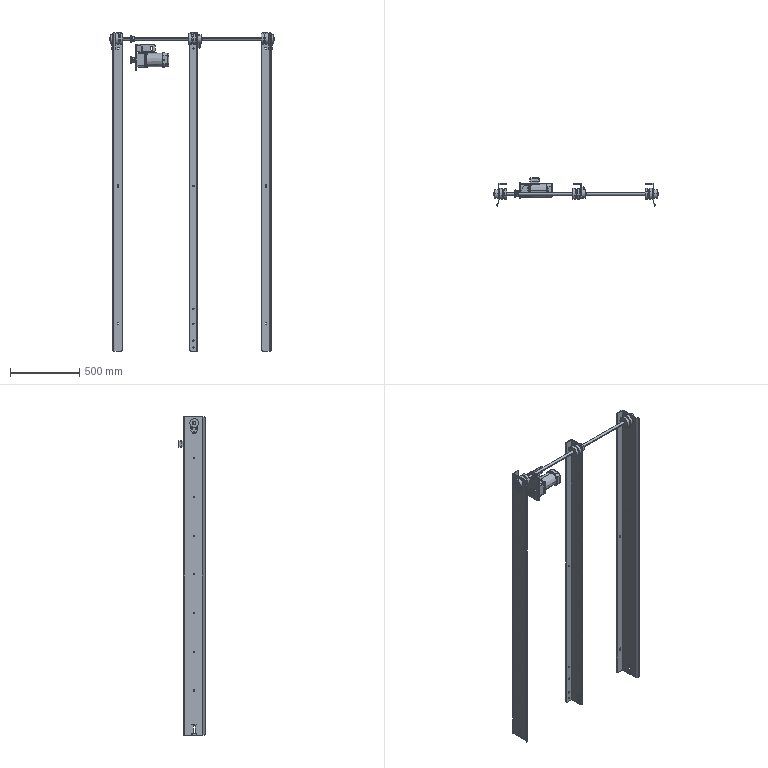Part | SolidWorks | features InContextFeatHolder 2, MirrorCompFeat 1, ReferencePattern 1 | 27 solids | 2410 faces | box 1198 x 199.551 x 2300 mm | volume 9436747 mm3 | cylinder 905 | plane 723 | spline 667 | cone 107 | torus 8 | commonest cylinder face diameters 8 x104 0.5 x64 3 x54 28.594 x52 9 x50 5 x48